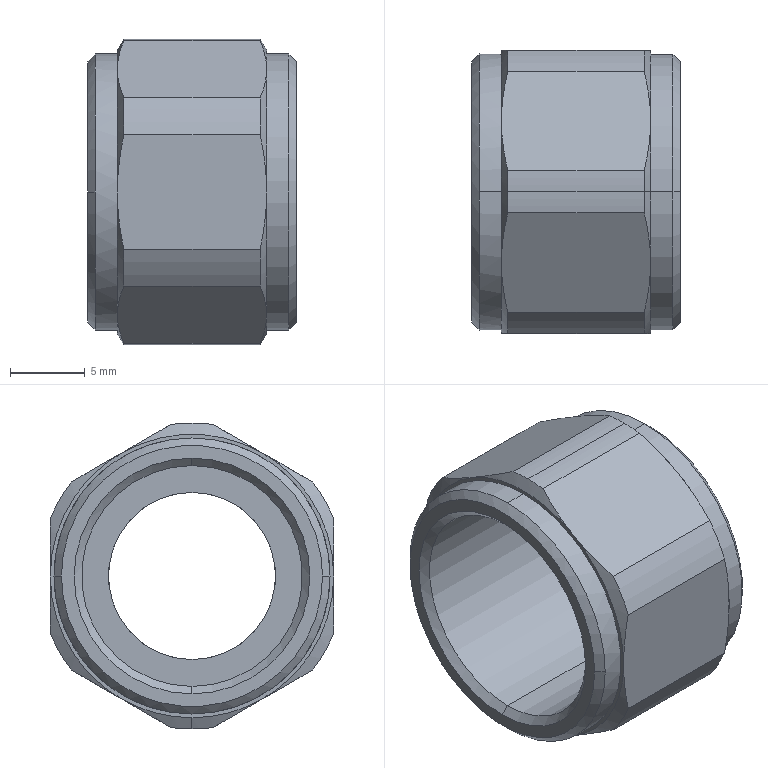Part | STEP file | 7C | 1 solid | 48 faces | box 14 x 19 x 20.5 mm | volume 1922 mm3 | cone 22 | cylinder 15 | plane 11 | commonest cylinder face diameters 20.5 x7 18.5 x4 11.2 x2 14.8 x2
STEP:
#1=CARTESIAN_POINT('',(11.,0.,-7.4));
#2=VERTEX_POINT('',#1);
#3=CARTESIAN_POINT('',(11.,0.,7.4));
#4=VERTEX_POINT('',#3);
#5=CARTESIAN_POINT('',(11.,0.,0.));
#6=DIRECTION('',(-1.,0.,0.));
#7=DIRECTION('',(0.,0.,1.));
#8=AXIS2_PLACEMENT_3D('',#5,#6,#7);
#9=CIRCLE('',#8,7.4);
#10=EDGE_CURVE('',#2,#4,#9,.T.);
#11=ORIENTED_EDGE('',*,*,#10,.F.);
#12=CARTESIAN_POINT('',(0.5,0.,-7.4));
#13=VERTEX_POINT('',#12);
#14=CARTESIAN_POINT('',(-2.908,0.,-7.4));
#15=DIRECTION('',(-1.,0.,0.));
#16=VECTOR('',#15,1000.);
#17=LINE('',#14,#16);
#18=EDGE_CURVE('',#2,#13,#17,.T.);
#19=ORIENTED_EDGE('',*,*,#18,.T.);
#20=CARTESIAN_POINT('',(0.5,0.,7.4));
#21=VERTEX_POINT('',#20);
#22=CARTESIAN_POINT('',(0.5,0.,0.));
#23=DIRECTION('',(1.,0.,0.));
#24=DIRECTION('',(0.,0.,1.));
#25=AXIS2_PLACEMENT_3D('',#22,#23,#24);
#26=CIRCLE('',#25,7.4);
#27=EDGE_CURVE('',#21,#13,#26,.T.);
#28=ORIENTED_EDGE('',*,*,#27,.F.);
#29=CARTESIAN_POINT('',(-2.908,0.,7.4));
#30=DIRECTION('',(-1.,0.,0.));
#31=VECTOR('',#30,1000.);
#32=LINE('',#29,#31);
#33=EDGE_CURVE('',#4,#21,#32,.T.);
#34=ORIENTED_EDGE('',*,*,#33,.F.);
#35=EDGE_LOOP('',(#11,#19,#28,#34));
#36=FACE_OUTER_BOUND('',#35,.T.);
#37=CARTESIAN_POINT('',(-2.908,0.,0.));
#38=DIRECTION('',(-1.,0.,0.));
#39=DIRECTION('',(0.,0.,1.));
#40=AXIS2_PLACEMENT_3D('',#37,#38,#39);
#41=CYLINDRICAL_SURFACE('',#40,7.4);
#42=ADVANCED_FACE('',(#36),#41,.F.);
#43=ORIENTED_EDGE('',*,*,#27,.T.);
#44=CARTESIAN_POINT('',(0.,0.,-7.9));
#45=VERTEX_POINT('',#44);
#46=CARTESIAN_POINT('',(0.,0.,-7.9));
#47=DIRECTION('',(-0.7071,0.,-0.7071));
#48=VECTOR('',#47,1000.);
#49=LINE('',#46,#48);
#50=EDGE_CURVE('',#13,#45,#49,.T.);
#51=ORIENTED_EDGE('',*,*,#50,.T.);
#52=CARTESIAN_POINT('',(0.,0.,7.9));
#53=VERTEX_POINT('',#52);
#54=CARTESIAN_POINT('',(0.,0.,0.));
#55=DIRECTION('',(1.,0.,0.));
#56=DIRECTION('',(0.,0.,1.));
#57=AXIS2_PLACEMENT_3D('',#54,#55,#56);
#58=CIRCLE('',#57,7.9);
#59=EDGE_CURVE('',#53,#45,#58,.T.);
#60=ORIENTED_EDGE('',*,*,#59,.F.);
#61=CARTESIAN_POINT('',(0.,0.,7.9));
#62=DIRECTION('',(-0.7071,0.,0.7071));
#63=VECTOR('',#62,1000.);
#64=LINE('',#61,#63);
#65=EDGE_CURVE('',#21,#53,#64,.T.);
#66=ORIENTED_EDGE('',*,*,#65,.F.);
#67=EDGE_LOOP('',(#43,#51,#60,#66));
#68=FACE_OUTER_BOUND('',#67,.T.);
#69=CARTESIAN_POINT('',(0.,0.,0.));
#70=DIRECTION('',(-1.,0.,0.));
#71=DIRECTION('',(0.,0.,1.));
#72=AXIS2_PLACEMENT_3D('',#69,#70,#71);
#73=CONICAL_SURFACE('',#72,7.9,0.7854);
#74=ADVANCED_FACE('',(#68),#73,.F.);
#75=CARTESIAN_POINT('',(13.5,0.,-5.6));
#76=VERTEX_POINT('',#75);
#77=CARTESIAN_POINT('',(13.5,-5.6,0.));
#78=VERTEX_POINT('',#77);
#79=CARTESIAN_POINT('',(13.5,0.,0.));
#80=DIRECTION('',(-1.,0.,0.));
#81=DIRECTION('',(0.,0.,1.));
#82=AXIS2_PLACEMENT_3D('',#79,#80,#81);
#83=CIRCLE('',#82,5.6);
#84=EDGE_CURVE('',#76,#78,#83,.T.);
#85=ORIENTED_EDGE('',*,*,#84,.F.);
#86=CARTESIAN_POINT('',(11.,0.,-5.6));
#87=VERTEX_POINT('',#86);
#88=CARTESIAN_POINT('',(-2.908,0.,-5.6));
#89=DIRECTION('',(-1.,0.,0.));
#90=VECTOR('',#89,1000.);
#91=LINE('',#88,#90);
#92=EDGE_CURVE('',#76,#87,#91,.T.);
#93=ORIENTED_EDGE('',*,*,#92,.T.);
#94=CARTESIAN_POINT('',(11.,0.,5.6));
#95=VERTEX_POINT('',#94);
#96=CARTESIAN_POINT('',(11.,0.,0.));
#97=DIRECTION('',(1.,0.,0.));
#98=DIRECTION('',(0.,0.,1.));
#99=AXIS2_PLACEMENT_3D('',#96,#97,#98);
#100=CIRCLE('',#99,5.6);
#101=EDGE_CURVE('',#95,#87,#100,.T.);
#102=ORIENTED_EDGE('',*,*,#101,.F.);
#103=CARTESIAN_POINT('',(13.5,0.,5.6));
#104=VERTEX_POINT('',#103);
#105=CARTESIAN_POINT('',(-2.908,0.,5.6));
#106=DIRECTION('',(-1.,0.,0.));
#107=VECTOR('',#106,1000.);
#108=LINE('',#105,#107);
#109=EDGE_CURVE('',#104,#95,#108,.T.);
#110=ORIENTED_EDGE('',*,*,#109,.F.);
#111=CARTESIAN_POINT('',(13.5,0.,0.));
#112=DIRECTION('',(-1.,0.,0.));
#113=DIRECTION('',(0.,0.,1.));
#114=AXIS2_PLACEMENT_3D('',#111,#112,#113);
#115=CIRCLE('',#114,5.6);
#116=EDGE_CURVE('',#78,#104,#115,.T.);
#117=ORIENTED_EDGE('',*,*,#116,.F.);
#118=EDGE_LOOP('',(#85,#93,#102,#110,#117));
#119=FACE_OUTER_BOUND('',#118,.T.);
#120=CARTESIAN_POINT('',(-2.908,0.,0.));
#121=DIRECTION('',(-1.,0.,0.));
#122=DIRECTION('',(0.,0.,1.));
#123=AXIS2_PLACEMENT_3D('',#120,#121,#122);
#124=CYLINDRICAL_SURFACE('',#123,5.6);
#125=ADVANCED_FACE('',(#119),#124,.F.);
#126=CARTESIAN_POINT('',(13.5,5.6,0.));
#127=VERTEX_POINT('',#126);
#128=CARTESIAN_POINT('',(13.5,0.,0.));
#129=DIRECTION('',(-1.,0.,0.));
#130=DIRECTION('',(0.,0.,1.));
#131=AXIS2_PLACEMENT_3D('',#128,#129,#130);
#132=CIRCLE('',#131,5.6);
#133=EDGE_CURVE('',#127,#76,#132,.T.);
#134=ORIENTED_EDGE('',*,*,#133,.T.);
#135=ORIENTED_EDGE('',*,*,#84,.T.);
#136=CARTESIAN_POINT('',(14.,-6.1,0.));
#137=VERTEX_POINT('',#136);
#138=CARTESIAN_POINT('',(14.,-6.1,0.));
#139=DIRECTION('',(0.7071,-0.7071,0.));
#140=VECTOR('',#139,1000.);
#141=LINE('',#138,#140);
#142=EDGE_CURVE('',#78,#137,#141,.T.);
#143=ORIENTED_EDGE('',*,*,#142,.T.);
#144=CARTESIAN_POINT('',(14.,6.1,0.));
#145=VERTEX_POINT('',#144);
#146=CARTESIAN_POINT('',(14.,0.,0.));
#147=DIRECTION('',(-1.,0.,0.));
#148=DIRECTION('',(0.,1.,0.));
#149=AXIS2_PLACEMENT_3D('',#146,#147,#148);
#150=CIRCLE('',#149,6.1);
#151=EDGE_CURVE('',#145,#137,#150,.T.);
#152=ORIENTED_EDGE('',*,*,#151,.F.);
#153=CARTESIAN_POINT('',(14.,6.1,0.));
#154=DIRECTION('',(0.7071,0.7071,0.));
#155=VECTOR('',#154,1000.);
#156=LINE('',#153,#155);
#157=EDGE_CURVE('',#127,#145,#156,.T.);
#158=ORIENTED_EDGE('',*,*,#157,.F.);
#159=EDGE_LOOP('',(#134,#135,#143,#152,#158));
#160=FACE_OUTER_BOUND('',#159,.T.);
#161=CARTESIAN_POINT('',(14.,0.,0.));
#162=DIRECTION('',(1.,0.,0.));
#163=DIRECTION('',(0.,1.,0.));
#164=AXIS2_PLACEMENT_3D('',#161,#162,#163);
#165=CONICAL_SURFACE('',#164,6.1,0.7854);
#166=ADVANCED_FACE('',(#160),#165,.F.);
#167=CARTESIAN_POINT('',(0.,8.75,0.));
#168=VERTEX_POINT('',#167);
#169=CARTESIAN_POINT('',(0.,-8.75,0.));
#170=VERTEX_POINT('',#169);
#171=CARTESIAN_POINT('',(0.,0.,0.));
#172=DIRECTION('',(1.,0.,0.));
#173=DIRECTION('',(0.,1.,0.));
#174=AXIS2_PLACEMENT_3D('',#171,#172,#173);
#175=CIRCLE('',#174,8.75);
#176=EDGE_CURVE('',#168,#170,#175,.T.);
#177=ORIENTED_EDGE('',*,*,#176,.T.);
#178=CARTESIAN_POINT('',(0.5,-9.25,0.));
#179=VERTEX_POINT('',#178);
#180=CARTESIAN_POINT('',(0.5,-9.25,0.));
#181=DIRECTION('',(0.7071,-0.7071,0.));
#182=VECTOR('',#181,1000.);
#183=LINE('',#180,#182);
#184=EDGE_CURVE('',#170,#179,#183,.T.);
#185=ORIENTED_EDGE('',*,*,#184,.T.);
#186=CARTESIAN_POINT('',(0.5,0.,9.25));
#187=VERTEX_POINT('',#186);
#188=CARTESIAN_POINT('',(0.5,0.,0.));
#189=DIRECTION('',(-1.,0.,0.));
#190=DIRECTION('',(0.,0.,-1.));
#191=AXIS2_PLACEMENT_3D('',#188,#189,#190);
#192=CIRCLE('',#191,9.25);
#193=EDGE_CURVE('',#179,#187,#192,.T.);
#194=ORIENTED_EDGE('',*,*,#193,.T.);
#195=CARTESIAN_POINT('',(0.5,9.25,0.));
#196=VERTEX_POINT('',#195);
#197=CARTESIAN_POINT('',(0.5,0.,0.));
#198=DIRECTION('',(-1.,0.,0.));
#199=DIRECTION('',(0.,0.,-1.));
#200=AXIS2_PLACEMENT_3D('',#197,#198,#199);
#201=CIRCLE('',#200,9.25);
#202=EDGE_CURVE('',#187,#196,#201,.T.);
#203=ORIENTED_EDGE('',*,*,#202,.T.);
#204=CARTESIAN_POINT('',(0.5,9.25,0.));
#205=DIRECTION('',(0.7071,0.7071,0.));
#206=VECTOR('',#205,1000.);
#207=LINE('',#204,#206);
#208=EDGE_CURVE('',#168,#196,#207,.T.);
#209=ORIENTED_EDGE('',*,*,#208,.F.);
#210=EDGE_LOOP('',(#177,#185,#194,#203,#209));
#211=FACE_OUTER_BOUND('',#210,.T.);
#212=CARTESIAN_POINT('',(0.5,0.,0.));
#213=DIRECTION('',(1.,0.,0.));
#214=DIRECTION('',(0.,1.,0.));
#215=AXIS2_PLACEMENT_3D('',#212,#213,#214);
#216=CONICAL_SURFACE('',#215,9.25,0.7854);
#217=ADVANCED_FACE('',(#211),#216,.T.);
#218=CARTESIAN_POINT('',(2.,0.,9.25));
#219=VERTEX_POINT('',#218);
#220=CARTESIAN_POINT('',(2.,0.,-9.25));
#221=VERTEX_POINT('',#220);
#222=CARTESIAN_POINT('',(2.,0.,0.));
#223=DIRECTION('',(-1.,0.,0.));
#224=DIRECTION('',(0.,0.,1.));
#225=AXIS2_PLACEMENT_3D('',#222,#223,#224);
#226=CIRCLE('',#225,9.25);
#227=EDGE_CURVE('',#219,#221,#226,.T.);
#228=ORIENTED_EDGE('',*,*,#227,.T.);
#229=CARTESIAN_POINT('',(0.5,0.,-9.25));
#230=VERTEX_POINT('',#229);
#231=CARTESIAN_POINT('',(-2.908,0.,-9.25));
#232=DIRECTION('',(-1.,0.,0.));
#233=VECTOR('',#232,1000.);
#234=LINE('',#231,#233);
#235=EDGE_CURVE('',#221,#230,#234,.T.);
#236=ORIENTED_EDGE('',*,*,#235,.T.);
#237=CARTESIAN_POINT('',(0.5,0.,0.));
#238=DIRECTION('',(-1.,0.,0.));
#239=DIRECTION('',(0.,0.,-1.));
#240=AXIS2_PLACEMENT_3D('',#237,#238,#239);
#241=CIRCLE('',#240,9.25);
#242=EDGE_CURVE('',#196,#230,#241,.T.);
#243=ORIENTED_EDGE('',*,*,#242,.F.);
#244=ORIENTED_EDGE('',*,*,#202,.F.);
#245=CARTESIAN_POINT('',(-2.908,0.,9.25));
#246=DIRECTION('',(-1.,0.,0.));
#247=VECTOR('',#246,1000.);
#248=LINE('',#245,#247);
#249=EDGE_CURVE('',#219,#187,#248,.T.);
#250=ORIENTED_EDGE('',*,*,#249,.F.);
#251=EDGE_LOOP('',(#228,#236,#243,#244,#250));
#252=FACE_OUTER_BOUND('',#251,.T.);
#253=CARTESIAN_POINT('',(-2.908,0.,0.));
#254=DIRECTION('',(-1.,0.,0.));
#255=DIRECTION('',(0.,0.,1.));
#256=AXIS2_PLACEMENT_3D('',#253,#254,#255);
#257=CYLINDRICAL_SURFACE('',#256,9.25);
#258=ADVANCED_FACE('',(#252),#257,.T.);
#259=CARTESIAN_POINT('',(14.,0.,-8.75));
#260=VERTEX_POINT('',#259);
#261=CARTESIAN_POINT('',(14.,0.,8.75));
#262=VERTEX_POINT('',#261);
#263=CARTESIAN_POINT('',(14.,0.,0.));
#264=DIRECTION('',(1.,0.,0.));
#265=DIRECTION('',(0.,0.,1.));
#266=AXIS2_PLACEMENT_3D('',#263,#264,#265);
#267=CIRCLE('',#266,8.75);
#268=EDGE_CURVE('',#260,#262,#267,.T.);
#269=ORIENTED_EDGE('',*,*,#268,.F.);
#270=CARTESIAN_POINT('',(13.5,0.,-9.25));
#271=VERTEX_POINT('',#270);
#272=CARTESIAN_POINT('',(13.5,0.,-9.25));
#273=DIRECTION('',(-0.7071,0.,-0.7071));
#274=VECTOR('',#273,1000.);
#275=LINE('',#272,#274);
#276=EDGE_CURVE('',#260,#271,#275,.T.);
#277=ORIENTED_EDGE('',*,*,#276,.T.);
#278=CARTESIAN_POINT('',(13.5,0.,9.25));
#279=VERTEX_POINT('',#278);
#280=CARTESIAN_POINT('',(13.5,0.,0.));
#281=DIRECTION('',(1.,0.,0.));
#282=DIRECTION('',(0.,0.,1.));
#283=AXIS2_PLACEMENT_3D('',#280,#281,#282);
#284=CIRCLE('',#283,9.25);
#285=EDGE_CURVE('',#271,#279,#284,.T.);
#286=ORIENTED_EDGE('',*,*,#285,.T.);
#287=CARTESIAN_POINT('',(13.5,0.,9.25));
#288=DIRECTION('',(-0.7071,0.,0.7071));
#289=VECTOR('',#288,1000.);
#290=LINE('',#287,#289);
#291=EDGE_CURVE('',#262,#279,#290,.T.);
#292=ORIENTED_EDGE('',*,*,#291,.F.);
#293=EDGE_LOOP('',(#269,#277,#286,#292));
#294=FACE_OUTER_BOUND('',#293,.T.);
#295=CARTESIAN_POINT('',(13.5,0.,0.));
#296=DIRECTION('',(-1.,0.,0.));
#297=DIRECTION('',(0.,0.,1.));
#298=AXIS2_PLACEMENT_3D('',#295,#296,#297);
#299=CONICAL_SURFACE('',#298,9.25,0.7854);
#300=ADVANCED_FACE('',(#294),#299,.T.);
#301=ORIENTED_EDGE('',*,*,#285,.F.);
#302=CARTESIAN_POINT('',(12.,0.,-9.25));
#303=VERTEX_POINT('',#302);
#304=CARTESIAN_POINT('',(-2.908,0.,-9.25));
#305=DIRECTION('',(-1.,0.,0.));
#306=VECTOR('',#305,1000.);
#307=LINE('',#304,#306);
#308=EDGE_CURVE('',#271,#303,#307,.T.);
#309=ORIENTED_EDGE('',*,*,#308,.T.);
#310=CARTESIAN_POINT('',(12.,0.,9.25));
#311=VERTEX_POINT('',#310);
#312=CARTESIAN_POINT('',(12.,0.,0.));
#313=DIRECTION('',(1.,0.,0.));
#314=DIRECTION('',(0.,0.,1.));
#315=AXIS2_PLACEMENT_3D('',#312,#313,#314);
#316=CIRCLE('',#315,9.25);
#317=EDGE_CURVE('',#303,#311,#316,.T.);
#318=ORIENTED_EDGE('',*,*,#317,.T.);
#319=CARTESIAN_POINT('',(-2.908,0.,9.25));
#320=DIRECTION('',(-1.,0.,0.));
#321=VECTOR('',#320,1000.);
#322=LINE('',#319,#321);
#323=EDGE_CURVE('',#279,#311,#322,.T.);
#324=ORIENTED_EDGE('',*,*,#323,.F.);
#325=EDGE_LOOP('',(#301,#309,#318,#324));
#326=FACE_OUTER_BOUND('',#325,.T.);
#327=CARTESIAN_POINT('',(-2.908,0.,0.));
#328=DIRECTION('',(-1.,0.,0.));
#329=DIRECTION('',(0.,0.,1.));
#330=AXIS2_PLACEMENT_3D('',#327,#328,#329);
#331=CYLINDRICAL_SURFACE('',#330,9.25);
#332=ADVANCED_FACE('',(#326),#331,.T.);
#333=CARTESIAN_POINT('',(2.,0.,-9.5));
#334=VERTEX_POINT('',#333);
#335=CARTESIAN_POINT('',(2.,-4.75,-8.227));
#336=VERTEX_POINT('',#335);
#337=CARTESIAN_POINT('',(2.,0.,0.));
#338=DIRECTION('',(-1.,0.,0.));
#339=DIRECTION('',(0.,0.,-1.));
#340=AXIS2_PLACEMENT_3D('',#337,#338,#339);
#341=CIRCLE('',#340,9.5);
#342=EDGE_CURVE('',#334,#336,#341,.T.);
#343=ORIENTED_EDGE('',*,*,#342,.F.);
#344=CARTESIAN_POINT('',(2.433,0.,-10.25));
#345=VERTEX_POINT('',#344);
#346=CARTESIAN_POINT('',(2.433,0.,-10.25));
#347=DIRECTION('',(0.5,0.,-0.866));
#348=VECTOR('',#347,1000.);
#349=LINE('',#346,#348);
#350=EDGE_CURVE('',#334,#345,#349,.T.);
#351=ORIENTED_EDGE('',*,*,#350,.T.);
#352=CARTESIAN_POINT('',(2.433,-1.417,-10.152));
#353=VERTEX_POINT('',#352);
#354=CARTESIAN_POINT('',(2.433,0.,0.));
#355=DIRECTION('',(1.,0.,0.));
#356=DIRECTION('',(0.,0.,1.));
#357=AXIS2_PLACEMENT_3D('',#354,#355,#356);
#358=CIRCLE('',#357,10.25);
#359=EDGE_CURVE('',#353,#345,#358,.T.);
#360=ORIENTED_EDGE('',*,*,#359,.F.);
#361=CARTESIAN_POINT('',(2.433,-1.417,-10.152));
#362=CARTESIAN_POINT('',(2.158,-2.515,-9.517));
#363=CARTESIAN_POINT('',(2.,-3.625,-8.877));
#364=CARTESIAN_POINT('',(2.,-4.75,-8.227));
#365=B_SPLINE_CURVE_WITH_KNOTS('',3,(#361,#362,#363,#364),.UNSPECIFIED.,.F.,.F.,(4,4),(0.,0.003873),.UNSPECIFIED.);
#366=EDGE_CURVE('',#353,#336,#365,.T.);
#367=ORIENTED_EDGE('',*,*,#366,.T.);
#368=EDGE_LOOP('',(#343,#351,#360,#367));
#369=FACE_OUTER_BOUND('',#368,.T.);
#370=CARTESIAN_POINT('',(2.433,0.,0.));
#371=DIRECTION('',(1.,0.,0.));
#372=DIRECTION('',(0.,0.,-1.));
#373=AXIS2_PLACEMENT_3D('',#370,#371,#372);
#374=CONICAL_SURFACE('',#373,10.25,1.047);
#375=ADVANCED_FACE('',(#369),#374,.T.);
#376=CARTESIAN_POINT('',(12.,0.,9.5));
#377=VERTEX_POINT('',#376);
#378=CARTESIAN_POINT('',(12.,-4.75,8.227));
#379=VERTEX_POINT('',#378);
#380=CARTESIAN_POINT('',(12.,0.,0.));
#381=DIRECTION('',(1.,0.,0.));
#382=DIRECTION('',(0.,0.,1.));
#383=AXIS2_PLACEMENT_3D('',#380,#381,#382);
#384=CIRCLE('',#383,9.5);
#385=EDGE_CURVE('',#377,#379,#384,.T.);
#386=ORIENTED_EDGE('',*,*,#385,.F.);
#387=CARTESIAN_POINT('',(11.567,0.,10.25));
#388=VERTEX_POINT('',#387);
#389=CARTESIAN_POINT('',(11.567,0.,10.25));
#390=DIRECTION('',(-0.5,0.,0.866));
#391=VECTOR('',#390,1000.);
#392=LINE('',#389,#391);
#393=EDGE_CURVE('',#377,#388,#392,.T.);
#394=ORIENTED_EDGE('',*,*,#393,.T.);
#395=CARTESIAN_POINT('',(11.567,-1.417,10.152));
#396=VERTEX_POINT('',#395);
#397=CARTESIAN_POINT('',(11.567,0.,0.));
#398=DIRECTION('',(1.,0.,0.));
#399=DIRECTION('',(0.,0.,1.));
#400=AXIS2_PLACEMENT_3D('',#397,#398,#399);
#401=CIRCLE('',#400,10.25);
#402=EDGE_CURVE('',#388,#396,#401,.T.);
#403=ORIENTED_EDGE('',*,*,#402,.T.);
#404=CARTESIAN_POINT('',(11.567,-1.417,10.152));
#405=CARTESIAN_POINT('',(11.842,-2.515,9.517));
#406=CARTESIAN_POINT('',(12.,-3.625,8.877));
#407=CARTESIAN_POINT('',(12.,-4.75,8.227));
#408=B_SPLINE_CURVE_WITH_KNOTS('',3,(#404,#405,#406,#407),.UNSPECIFIED.,.F.,.F.,(4,4),(0.,0.003873),.UNSPECIFIED.);
#409=EDGE_CURVE('',#396,#379,#408,.T.);
#410=ORIENTED_EDGE('',*,*,#409,.T.);
#411=EDGE_LOOP('',(#386,#394,#403,#410));
#412=FACE_OUTER_BOUND('',#411,.T.);
#413=CARTESIAN_POINT('',(11.567,0.,0.));
#414=DIRECTION('',(-1.,0.,0.));
#415=DIRECTION('',(0.,0.,1.));
#416=AXIS2_PLACEMENT_3D('',#413,#414,#415);
#417=CONICAL_SURFACE('',#416,10.25,1.047);
#418=ADVANCED_FACE('',(#412),#417,.T.);
#419=ORIENTED_EDGE('',*,*,#402,.F.);
#420=CARTESIAN_POINT('',(2.433,0.,10.25));
#421=VERTEX_POINT('',#420);
#422=CARTESIAN_POINT('',(-2.908,0.,10.25));
#423=DIRECTION('',(-1.,0.,0.));
#424=VECTOR('',#423,1000.);
#425=LINE('',#422,#424);
#426=EDGE_CURVE('',#388,#421,#425,.T.);
#427=ORIENTED_EDGE('',*,*,#426,.T.);
#428=CARTESIAN_POINT('',(2.433,-1.417,10.152));
#429=VERTEX_POINT('',#428);
#430=CARTESIAN_POINT('',(2.433,0.,0.));
#431=DIRECTION('',(1.,0.,0.));
#432=DIRECTION('',(0.,0.,1.));
#433=AXIS2_PLACEMENT_3D('',#430,#431,#432);
#434=CIRCLE('',#433,10.25);
#435=EDGE_CURVE('',#421,#429,#434,.T.);
#436=ORIENTED_EDGE('',*,*,#435,.T.);
#437=CARTESIAN_POINT('',(14.,-1.417,10.152));
#438=DIRECTION('',(1.,0.,0.));
#439=VECTOR('',#438,1000.);
#440=LINE('',#437,#439);
#441=EDGE_CURVE('',#429,#396,#440,.T.);
#442=ORIENTED_EDGE('',*,*,#441,.T.);
#443=EDGE_LOOP('',(#419,#427,#436,#442));
#444=FACE_OUTER_BOUND('',#443,.T.);
#445=CARTESIAN_POINT('',(-2.908,0.,0.));
#446=DIRECTION('',(-1.,0.,0.));
#447=DIRECTION('',(0.,0.,1.));
#448=AXIS2_PLACEMENT_3D('',#445,#446,#447);
#449=CYLINDRICAL_SURFACE('',#448,10.25);
#450=ADVANCED_FACE('',(#444),#449,.T.);
#451=ORIENTED_EDGE('',*,*,#18,.F.);
#452=CARTESIAN_POINT('',(11.,0.,0.));
#453=DIRECTION('',(-1.,0.,0.));
#454=DIRECTION('',(0.,0.,1.));
#455=AXIS2_PLACEMENT_3D('',#452,#453,#454);
#456=CIRCLE('',#455,7.4);
#457=EDGE_CURVE('',#4,#2,#456,.T.);
#458=ORIENTED_EDGE('',*,*,#457,.F.);
#459=ORIENTED_EDGE('',*,*,#33,.T.);
#460=CARTESIAN_POINT('',(0.5,0.,0.));
#461=DIRECTION('',(1.,0.,0.));
#462=DIRECTION('',(0.,0.,1.));
#463=AXIS2_PLACEMENT_3D('',#460,#461,#462);
#464=CIRCLE('',#463,7.4);
#465=EDGE_CURVE('',#13,#21,#464,.T.);
#466=ORIENTED_EDGE('',*,*,#465,.F.);
#467=EDGE_LOOP('',(#451,#458,#459,#466));
#468=FACE_OUTER_BOUND('',#467,.T.);
#469=CARTESIAN_POINT('',(-2.908,0.,0.));
#470=DIRECTION('',(-1.,0.,0.));
#471=DIRECTION('',(0.,0.,1.));
#472=AXIS2_PLACEMENT_3D('',#469,#470,#471);
#473=CYLINDRICAL_SURFACE('',#472,7.4);
#474=ADVANCED_FACE('',(#468),#473,.F.);
#475=ORIENTED_EDGE('',*,*,#101,.T.);
#476=CARTESIAN_POINT('',(11.,0.,0.));
#477=DIRECTION('',(1.,0.,0.));
#478=DIRECTION('',(0.,0.,1.));
#479=AXIS2_PLACEMENT_3D('',#476,#477,#478);
#480=CIRCLE('',#479,5.6);
#481=EDGE_CURVE('',#87,#95,#480,.T.);
#482=ORIENTED_EDGE('',*,*,#481,.T.);
#483=EDGE_LOOP('',(#475,#482));
#484=FACE_BOUND('',#483,.T.);
#485=ORIENTED_EDGE('',*,*,#457,.T.);
#486=ORIENTED_EDGE('',*,*,#10,.T.);
#487=EDGE_LOOP('',(#485,#486));
#488=FACE_OUTER_BOUND('',#487,.T.);
#489=CARTESIAN_POINT('',(11.,0.,-7.4));
#490=DIRECTION('',(-1.,0.,0.));
#491=DIRECTION('',(0.,0.,1.));
#492=AXIS2_PLACEMENT_3D('',#489,#490,#491);
#493=PLANE('',#492);
#494=ADVANCED_FACE('',(#484,#488),#493,.T.);
#495=ORIENTED_EDGE('',*,*,#50,.F.);
#496=ORIENTED_EDGE('',*,*,#465,.T.);
#497=ORIENTED_EDGE('',*,*,#65,.T.);
#498=CARTESIAN_POINT('',(0.,0.,0.));
#499=DIRECTION('',(1.,0.,0.));
#500=DIRECTION('',(0.,0.,1.));
#501=AXIS2_PLACEMENT_3D('',#498,#499,#500);
#502=CIRCLE('',#501,7.9);
#503=EDGE_CURVE('',#45,#53,#502,.T.);
#504=ORIENTED_EDGE('',*,*,#503,.F.);
#505=EDGE_LOOP('',(#495,#496,#497,#504));
#506=FACE_OUTER_BOUND('',#505,.T.);
#507=CARTESIAN_POINT('',(0.,0.,0.));
#508=DIRECTION('',(-1.,0.,0.));
#509=DIRECTION('',(0.,0.,1.));
#510=AXIS2_PLACEMENT_3D('',#507,#508,#509);
#511=CONICAL_SURFACE('',#510,7.9,0.7854);
#512=ADVANCED_FACE('',(#506),#511,.F.);
#513=ORIENTED_EDGE('',*,*,#92,.F.);
#514=ORIENTED_EDGE('',*,*,#133,.F.);
#515=CARTESIAN_POINT('',(13.5,0.,0.));
#516=DIRECTION('',(-1.,0.,0.));
#517=DIRECTION('',(0.,0.,1.));
#518=AXIS2_PLACEMENT_3D('',#515,#516,#517);
#519=CIRCLE('',#518,5.6);
#520=EDGE_CURVE('',#104,#127,#519,.T.);
#521=ORIENTED_EDGE('',*,*,#520,.F.);
#522=ORIENTED_EDGE('',*,*,#109,.T.);
#523=ORIENTED_EDGE('',*,*,#481,.F.);
#524=EDGE_LOOP('',(#513,#514,#521,#522,#523));
#525=FACE_OUTER_BOUND('',#524,.T.);
#526=CARTESIAN_POINT('',(-2.908,0.,0.));
#527=DIRECTION('',(-1.,0.,0.));
#528=DIRECTION('',(0.,0.,1.));
#529=AXIS2_PLACEMENT_3D('',#526,#527,#528);
#530=CYLINDRICAL_SURFACE('',#529,5.6);
#531=ADVANCED_FACE('',(#525),#530,.F.);
#532=ORIENTED_EDGE('',*,*,#59,.T.);
#533=ORIENTED_EDGE('',*,*,#503,.T.);
#534=EDGE_LOOP('',(#532,#533));
#535=FACE_BOUND('',#534,.T.);
#536=ORIENTED_EDGE('',*,*,#176,.F.);
#537=CARTESIAN_POINT('',(0.,0.,0.));
#538=DIRECTION('',(1.,0.,0.));
#539=DIRECTION('',(0.,1.,0.));
#540=AXIS2_PLACEMENT_3D('',#537,#538,#539);
#541=CIRCLE('',#540,8.75);
#542=EDGE_CURVE('',#170,#168,#541,.T.);
#543=ORIENTED_EDGE('',*,*,#542,.F.);
#544=EDGE_LOOP('',(#536,#543));
#545=FACE_OUTER_BOUND('',#544,.T.);
#546=CARTESIAN_POINT('',(0.,0.,-10.97));
#547=DIRECTION('',(1.,0.,0.));
#548=DIRECTION('',(0.,0.,-1.));
#549=AXIS2_PLACEMENT_3D('',#546,#547,#548);
#550=PLANE('',#549);
#551=ADVANCED_FACE('',(#535,#545),#550,.F.);
#552=ORIENTED_EDGE('',*,*,#142,.F.);
#553=ORIENTED_EDGE('',*,*,#116,.T.);
#554=ORIENTED_EDGE('',*,*,#520,.T.);
#555=ORIENTED_EDGE('',*,*,#157,.T.);
#556=CARTESIAN_POINT('',(14.,0.,0.));
#557=DIRECTION('',(-1.,0.,0.));
#558=DIRECTION('',(0.,1.,0.));
#559=AXIS2_PLACEMENT_3D('',#556,#557,#558);
#560=CIRCLE('',#559,6.1);
#561=EDGE_CURVE('',#137,#145,#560,.T.);
#562=ORIENTED_EDGE('',*,*,#561,.F.);
#563=EDGE_LOOP('',(#552,#553,#554,#555,#562));
#564=FACE_OUTER_BOUND('',#563,.T.);
#565=CARTESIAN_POINT('',(14.,0.,0.));
#566=DIRECTION('',(1.,0.,0.));
#567=DIRECTION('',(0.,1.,0.));
#568=AXIS2_PLACEMENT_3D('',#565,#566,#567);
#569=CONICAL_SURFACE('',#568,6.1,0.7854);
#570=ADVANCED_FACE('',(#564),#569,.F.);
#571=ORIENTED_EDGE('',*,*,#184,.F.);
#572=ORIENTED_EDGE('',*,*,#542,.T.);
#573=ORIENTED_EDGE('',*,*,#208,.T.);
#574=ORIENTED_EDGE('',*,*,#242,.T.);
#575=CARTESIAN_POINT('',(0.5,0.,0.));
#576=DIRECTION('',(-1.,0.,0.));
#577=DIRECTION('',(0.,0.,-1.));
#578=AXIS2_PLACEMENT_3D('',#575,#576,#577);
#579=CIRCLE('',#578,9.25);
#580=EDGE_CURVE('',#230,#179,#579,.T.);
#581=ORIENTED_EDGE('',*,*,#580,.T.);
#582=EDGE_LOOP('',(#571,#572,#573,#574,#581));
#583=FACE_OUTER_BOUND('',#582,.T.);
#584=CARTESIAN_POINT('',(0.5,0.,0.));
#585=DIRECTION('',(1.,0.,0.));
#586=DIRECTION('',(0.,1.,0.));
#587=AXIS2_PLACEMENT_3D('',#584,#585,#586);
#588=CONICAL_SURFACE('',#587,9.25,0.7854);
#589=ADVANCED_FACE('',(#583),#588,.T.);
#590=CARTESIAN_POINT('',(14.,0.,0.));
#591=DIRECTION('',(1.,0.,0.));
#592=DIRECTION('',(0.,0.,1.));
#593=AXIS2_PLACEMENT_3D('',#590,#591,#592);
#594=CIRCLE('',#593,8.75);
#595=EDGE_CURVE('',#262,#260,#594,.T.);
#596=ORIENTED_EDGE('',*,*,#595,.T.);
#597=ORIENTED_EDGE('',*,*,#268,.T.);
#598=EDGE_LOOP('',(#596,#597));
#599=FACE_OUTER_BOUND('',#598,.T.);
#600=ORIENTED_EDGE('',*,*,#151,.T.);
#601=ORIENTED_EDGE('',*,*,#561,.T.);
#602=EDGE_LOOP('',(#600,#601));
#603=FACE_BOUND('',#602,.T.);
#604=CARTESIAN_POINT('',(14.,0.,-10.97));
#605=DIRECTION('',(1.,0.,0.));
#606=DIRECTION('',(0.,0.,-1.));
#607=AXIS2_PLACEMENT_3D('',#604,#605,#606);
#608=PLANE('',#607);
#609=ADVANCED_FACE('',(#599,#603),#608,.T.);
#610=ORIENTED_EDGE('',*,*,#235,.F.);
#611=CARTESIAN_POINT('',(2.,0.,0.));
#612=DIRECTION('',(-1.,0.,0.));
#613=DIRECTION('',(0.,0.,1.));
#614=AXIS2_PLACEMENT_3D('',#611,#612,#613);
#615=CIRCLE('',#614,9.25);
#616=EDGE_CURVE('',#221,#219,#615,.T.);
#617=ORIENTED_EDGE('',*,*,#616,.T.);
#618=ORIENTED_EDGE('',*,*,#249,.T.);
#619=ORIENTED_EDGE('',*,*,#193,.F.);
#620=ORIENTED_EDGE('',*,*,#580,.F.);
#621=EDGE_LOOP('',(#610,#617,#618,#619,#620));
#622=FACE_OUTER_BOUND('',#621,.T.);
#623=CARTESIAN_POINT('',(-2.908,0.,0.));
#624=DIRECTION('',(-1.,0.,0.));
#625=DIRECTION('',(0.,0.,1.));
#626=AXIS2_PLACEMENT_3D('',#623,#624,#625);
#627=CYLINDRICAL_SURFACE('',#626,9.25);
#628=ADVANCED_FACE('',(#622),#627,.T.);
#629=ORIENTED_EDGE('',*,*,#276,.F.);
#630=ORIENTED_EDGE('',*,*,#595,.F.);
#631=ORIENTED_EDGE('',*,*,#291,.T.);
#632=CARTESIAN_POINT('',(13.5,0.,0.));
#633=DIRECTION('',(1.,0.,0.));
#634=DIRECTION('',(0.,0.,1.));
#635=AXIS2_PLACEMENT_3D('',#632,#633,#634);
#636=CIRCLE('',#635,9.25);
#637=EDGE_CURVE('',#279,#271,#636,.T.);
#638=ORIENTED_EDGE('',*,*,#637,.T.);
#639=EDGE_LOOP('',(#629,#630,#631,#638));
#640=FACE_OUTER_BOUND('',#639,.T.);
#641=CARTESIAN_POINT('',(13.5,0.,0.));
#642=DIRECTION('',(-1.,0.,0.));
#643=DIRECTION('',(0.,0.,1.));
#644=AXIS2_PLACEMENT_3D('',#641,#642,#643);
#645=CONICAL_SURFACE('',#644,9.25,0.7854);
#646=ADVANCED_FACE('',(#640),#645,.T.);
#647=ORIENTED_EDGE('',*,*,#227,.F.);
#648=ORIENTED_EDGE('',*,*,#616,.F.);
#649=EDGE_LOOP('',(#647,#648));
#650=FACE_BOUND('',#649,.T.);
#651=CARTESIAN_POINT('',(2.,-9.5,0.));
#652=VERTEX_POINT('',#651);
#653=CARTESIAN_POINT('',(2.,-4.75,8.227));
#654=VERTEX_POINT('',#653);
#655=CARTESIAN_POINT('',(2.,0.,0.));
#656=DIRECTION('',(-1.,0.,0.));
#657=DIRECTION('',(0.,0.,-1.));
#658=AXIS2_PLACEMENT_3D('',#655,#656,#657);
#659=CIRCLE('',#658,9.5);
#660=EDGE_CURVE('',#652,#654,#659,.T.);
#661=ORIENTED_EDGE('',*,*,#660,.T.);
#662=CARTESIAN_POINT('',(2.,4.75,8.227));
#663=VERTEX_POINT('',#662);
#664=CARTESIAN_POINT('',(2.,0.,0.));
#665=DIRECTION('',(-1.,0.,0.));
#666=DIRECTION('',(0.,0.,-1.));
#667=AXIS2_PLACEMENT_3D('',#664,#665,#666);
#668=CIRCLE('',#667,9.5);
#669=EDGE_CURVE('',#654,#663,#668,.T.);
#670=ORIENTED_EDGE('',*,*,#669,.T.);
#671=CARTESIAN_POINT('',(2.,9.5,0.));
#672=VERTEX_POINT('',#671);
#673=CARTESIAN_POINT('',(2.,0.,0.));
#674=DIRECTION('',(-1.,0.,0.));
#675=DIRECTION('',(0.,0.,-1.));
#676=AXIS2_PLACEMENT_3D('',#673,#674,#675);
#677=CIRCLE('',#676,9.5);
#678=EDGE_CURVE('',#663,#672,#677,.T.);
#679=ORIENTED_EDGE('',*,*,#678,.T.);
#680=CARTESIAN_POINT('',(2.,4.75,-8.227));
#681=VERTEX_POINT('',#680);
#682=CARTESIAN_POINT('',(2.,0.,0.));
#683=DIRECTION('',(-1.,0.,0.));
#684=DIRECTION('',(0.,0.,-1.));
#685=AXIS2_PLACEMENT_3D('',#682,#683,#684);
#686=CIRCLE('',#685,9.5);
#687=EDGE_CURVE('',#672,#681,#686,.T.);
#688=ORIENTED_EDGE('',*,*,#687,.T.);
#689=CARTESIAN_POINT('',(2.,0.,0.));
#690=DIRECTION('',(-1.,0.,0.));
#691=DIRECTION('',(0.,0.,-1.));
#692=AXIS2_PLACEMENT_3D('',#689,#690,#691);
#693=CIRCLE('',#692,9.5);
#694=EDGE_CURVE('',#681,#334,#693,.T.);
#695=ORIENTED_EDGE('',*,*,#694,.T.);
#696=ORIENTED_EDGE('',*,*,#342,.T.);
#697=CARTESIAN_POINT('',(2.,0.,0.));
#698=DIRECTION('',(-1.,0.,0.));
#699=DIRECTION('',(0.,0.,-1.));
#700=AXIS2_PLACEMENT_3D('',#697,#698,#699);
#701=CIRCLE('',#700,9.5);
#702=EDGE_CURVE('',#336,#652,#701,.T.);
#703=ORIENTED_EDGE('',*,*,#702,.T.);
#704=EDGE_LOOP('',(#661,#670,#679,#688,#695,#696,#703));
#705=FACE_OUTER_BOUND('',#704,.T.);
#706=CARTESIAN_POINT('',(2.,0.,-9.25));
#707=DIRECTION('',(-1.,0.,0.));
#708=DIRECTION('',(0.,0.,1.));
#709=AXIS2_PLACEMENT_3D('',#706,#707,#708);
#710=PLANE('',#709);
#711=ADVANCED_FACE('',(#650,#705),#710,.T.);
#712=ORIENTED_EDGE('',*,*,#308,.F.);
#713=ORIENTED_EDGE('',*,*,#637,.F.);
#714=ORIENTED_EDGE('',*,*,#323,.T.);
#715=CARTESIAN_POINT('',(12.,0.,0.));
#716=DIRECTION('',(1.,0.,0.));
#717=DIRECTION('',(0.,0.,1.));
#718=AXIS2_PLACEMENT_3D('',#715,#716,#717);
#719=CIRCLE('',#718,9.25);
#720=EDGE_CURVE('',#311,#303,#719,.T.);
#721=ORIENTED_EDGE('',*,*,#720,.T.);
#722=EDGE_LOOP('',(#712,#713,#714,#721));
#723=FACE_OUTER_BOUND('',#722,.T.);
#724=CARTESIAN_POINT('',(-2.908,0.,0.));
#725=DIRECTION('',(-1.,0.,0.));
#726=DIRECTION('',(0.,0.,1.));
#727=AXIS2_PLACEMENT_3D('',#724,#725,#726);
#728=CYLINDRICAL_SURFACE('',#727,9.25);
#729=ADVANCED_FACE('',(#723),#728,.T.);
#730=CARTESIAN_POINT('',(2.433,1.417,10.152));
#731=VERTEX_POINT('',#730);
#732=CARTESIAN_POINT('',(2.433,0.,0.));
#733=DIRECTION('',(1.,0.,0.));
#734=DIRECTION('',(0.,0.,1.));
#735=AXIS2_PLACEMENT_3D('',#732,#733,#734);
#736=CIRCLE('',#735,10.25);
#737=EDGE_CURVE('',#731,#421,#736,.T.);
#738=ORIENTED_EDGE('',*,*,#737,.F.);
#739=CARTESIAN_POINT('',(2.433,1.417,10.152));
#740=CARTESIAN_POINT('',(2.158,2.515,9.517));
#741=CARTESIAN_POINT('',(2.,3.625,8.877));
#742=CARTESIAN_POINT('',(2.,4.75,8.227));
#743=B_SPLINE_CURVE_WITH_KNOTS('',3,(#739,#740,#741,#742),.UNSPECIFIED.,.F.,.F.,(4,4),(0.,0.003873),.UNSPECIFIED.);
#744=EDGE_CURVE('',#731,#663,#743,.T.);
#745=ORIENTED_EDGE('',*,*,#744,.T.);
#746=ORIENTED_EDGE('',*,*,#669,.F.);
#747=CARTESIAN_POINT('',(2.,-4.75,8.227));
#748=CARTESIAN_POINT('',(2.,-3.625,8.877));
#749=CARTESIAN_POINT('',(2.158,-2.515,9.517));
#750=CARTESIAN_POINT('',(2.433,-1.417,10.152));
#751=B_SPLINE_CURVE_WITH_KNOTS('',3,(#747,#748,#749,#750),.UNSPECIFIED.,.F.,.F.,(4,4),(0.,0.003873),.UNSPECIFIED.);
#752=EDGE_CURVE('',#654,#429,#751,.T.);
#753=ORIENTED_EDGE('',*,*,#752,.T.);
#754=ORIENTED_EDGE('',*,*,#435,.F.);
#755=EDGE_LOOP('',(#738,#745,#746,#753,#754));
#756=FACE_OUTER_BOUND('',#755,.T.);
#757=CARTESIAN_POINT('',(2.433,0.,0.));
#758=DIRECTION('',(1.,0.,0.));
#759=DIRECTION('',(0.,0.,-1.));
#760=AXIS2_PLACEMENT_3D('',#757,#758,#759);
#761=CONICAL_SURFACE('',#760,10.25,1.047);
#762=ADVANCED_FACE('',(#756),#761,.T.);
#763=CARTESIAN_POINT('',(2.433,-9.5,3.849));
#764=VERTEX_POINT('',#763);
#765=CARTESIAN_POINT('',(2.,-9.5,0.));
#766=CARTESIAN_POINT('',(2.,-9.5,1.299));
#767=CARTESIAN_POINT('',(2.158,-9.5,2.58));
#768=CARTESIAN_POINT('',(2.433,-9.5,3.849));
#769=B_SPLINE_CURVE_WITH_KNOTS('',3,(#765,#766,#767,#768),.UNSPECIFIED.,.F.,.F.,(4,4),(0.,0.003873),.UNSPECIFIED.);
#770=EDGE_CURVE('',#652,#764,#769,.T.);
#771=ORIENTED_EDGE('',*,*,#770,.T.);
#772=CARTESIAN_POINT('',(2.433,-8.083,6.303));
#773=VERTEX_POINT('',#772);
#774=CARTESIAN_POINT('',(2.433,0.,0.));
#775=DIRECTION('',(-1.,0.,0.));
#776=DIRECTION('',(0.,0.,-1.));
#777=AXIS2_PLACEMENT_3D('',#774,#775,#776);
#778=CIRCLE('',#777,10.25);
#779=EDGE_CURVE('',#764,#773,#778,.T.);
#780=ORIENTED_EDGE('',*,*,#779,.T.);
#781=CARTESIAN_POINT('',(2.433,-8.083,6.303));
#782=CARTESIAN_POINT('',(2.158,-6.985,6.937));
#783=CARTESIAN_POINT('',(2.,-5.875,7.578));
#784=CARTESIAN_POINT('',(2.,-4.75,8.227));
#785=B_SPLINE_CURVE_WITH_KNOTS('',3,(#781,#782,#783,#784),.UNSPECIFIED.,.F.,.F.,(4,4),(0.,0.003873),.UNSPECIFIED.);
#786=EDGE_CURVE('',#773,#654,#785,.T.);
#787=ORIENTED_EDGE('',*,*,#786,.T.);
#788=ORIENTED_EDGE('',*,*,#660,.F.);
#789=EDGE_LOOP('',(#771,#780,#787,#788));
#790=FACE_OUTER_BOUND('',#789,.T.);
#791=CARTESIAN_POINT('',(2.433,0.,0.));
#792=DIRECTION('',(1.,0.,0.));
#793=DIRECTION('',(0.,0.,-1.));
#794=AXIS2_PLACEMENT_3D('',#791,#792,#793);
#795=CONICAL_SURFACE('',#794,10.25,1.047);
#796=ADVANCED_FACE('',(#790),#795,.T.);
#797=CARTESIAN_POINT('',(2.433,-9.5,-3.849));
#798=VERTEX_POINT('',#797);
#799=CARTESIAN_POINT('',(2.433,-9.5,-3.849));
#800=CARTESIAN_POINT('',(2.158,-9.5,-2.58));
#801=CARTESIAN_POINT('',(2.,-9.5,-1.299));
#802=CARTESIAN_POINT('',(2.,-9.5,0.));
#803=B_SPLINE_CURVE_WITH_KNOTS('',3,(#799,#800,#801,#802),.UNSPECIFIED.,.F.,.F.,(4,4),(0.,0.003873),.UNSPECIFIED.);
#804=EDGE_CURVE('',#798,#652,#803,.T.);
#805=ORIENTED_EDGE('',*,*,#804,.T.);
#806=ORIENTED_EDGE('',*,*,#702,.F.);
#807=CARTESIAN_POINT('',(2.433,-8.083,-6.303));
#808=VERTEX_POINT('',#807);
#809=CARTESIAN_POINT('',(2.,-4.75,-8.227));
#810=CARTESIAN_POINT('',(2.,-5.875,-7.578));
#811=CARTESIAN_POINT('',(2.158,-6.985,-6.937));
#812=CARTESIAN_POINT('',(2.433,-8.083,-6.303));
#813=B_SPLINE_CURVE_WITH_KNOTS('',3,(#809,#810,#811,#812),.UNSPECIFIED.,.F.,.F.,(4,4),(0.,0.003873),.UNSPECIFIED.);
#814=EDGE_CURVE('',#336,#808,#813,.T.);
#815=ORIENTED_EDGE('',*,*,#814,.T.);
#816=CARTESIAN_POINT('',(2.433,0.,0.));
#817=DIRECTION('',(-1.,0.,0.));
#818=DIRECTION('',(0.,0.,-1.));
#819=AXIS2_PLACEMENT_3D('',#816,#817,#818);
#820=CIRCLE('',#819,10.25);
#821=EDGE_CURVE('',#808,#798,#820,.T.);
#822=ORIENTED_EDGE('',*,*,#821,.T.);
#823=EDGE_LOOP('',(#805,#806,#815,#822));
#824=FACE_OUTER_BOUND('',#823,.T.);
#825=CARTESIAN_POINT('',(2.433,0.,0.));
#826=DIRECTION('',(1.,0.,0.));
#827=DIRECTION('',(0.,0.,-1.));
#828=AXIS2_PLACEMENT_3D('',#825,#826,#827);
#829=CONICAL_SURFACE('',#828,10.25,1.047);
#830=ADVANCED_FACE('',(#824),#829,.T.);
#831=ORIENTED_EDGE('',*,*,#350,.F.);
#832=ORIENTED_EDGE('',*,*,#694,.F.);
#833=CARTESIAN_POINT('',(2.433,1.417,-10.152));
#834=VERTEX_POINT('',#833);
#835=CARTESIAN_POINT('',(2.,4.75,-8.227));
#836=CARTESIAN_POINT('',(2.,3.625,-8.877));
#837=CARTESIAN_POINT('',(2.158,2.515,-9.517));
#838=CARTESIAN_POINT('',(2.433,1.417,-10.152));
#839=B_SPLINE_CURVE_WITH_KNOTS('',3,(#835,#836,#837,#838),.UNSPECIFIED.,.F.,.F.,(4,4),(0.,0.003873),.UNSPECIFIED.);
#840=EDGE_CURVE('',#681,#834,#839,.T.);
#841=ORIENTED_EDGE('',*,*,#840,.T.);
#842=CARTESIAN_POINT('',(2.433,0.,0.));
#843=DIRECTION('',(1.,0.,0.));
#844=DIRECTION('',(0.,0.,1.));
#845=AXIS2_PLACEMENT_3D('',#842,#843,#844);
#846=CIRCLE('',#845,10.25);
#847=EDGE_CURVE('',#345,#834,#846,.T.);
#848=ORIENTED_EDGE('',*,*,#847,.F.);
#849=EDGE_LOOP('',(#831,#832,#841,#848));
#850=FACE_OUTER_BOUND('',#849,.T.);
#851=CARTESIAN_POINT('',(2.433,0.,0.));
#852=DIRECTION('',(1.,0.,0.));
#853=DIRECTION('',(0.,0.,-1.));
#854=AXIS2_PLACEMENT_3D('',#851,#852,#853);
#855=CONICAL_SURFACE('',#854,10.25,1.047);
#856=ADVANCED_FACE('',(#850),#855,.T.);
#857=CARTESIAN_POINT('',(2.433,9.5,-3.849));
#858=VERTEX_POINT('',#857);
#859=CARTESIAN_POINT('',(2.,9.5,0.));
#860=CARTESIAN_POINT('',(2.,9.5,-1.299));
#861=CARTESIAN_POINT('',(2.158,9.5,-2.58));
#862=CARTESIAN_POINT('',(2.433,9.5,-3.849));
#863=B_SPLINE_CURVE_WITH_KNOTS('',3,(#859,#860,#861,#862),.UNSPECIFIED.,.F.,.F.,(4,4),(0.,0.003873),.UNSPECIFIED.);
#864=EDGE_CURVE('',#672,#858,#863,.T.);
#865=ORIENTED_EDGE('',*,*,#864,.T.);
#866=CARTESIAN_POINT('',(2.433,8.083,-6.303));
#867=VERTEX_POINT('',#866);
#868=CARTESIAN_POINT('',(2.433,0.,0.));
#869=DIRECTION('',(-1.,0.,0.));
#870=DIRECTION('',(0.,0.,-1.));
#871=AXIS2_PLACEMENT_3D('',#868,#869,#870);
#872=CIRCLE('',#871,10.25);
#873=EDGE_CURVE('',#858,#867,#872,.T.);
#874=ORIENTED_EDGE('',*,*,#873,.T.);
#875=CARTESIAN_POINT('',(2.433,8.083,-6.303));
#876=CARTESIAN_POINT('',(2.158,6.985,-6.937));
#877=CARTESIAN_POINT('',(2.,5.875,-7.578));
#878=CARTESIAN_POINT('',(2.,4.75,-8.227));
#879=B_SPLINE_CURVE_WITH_KNOTS('',3,(#875,#876,#877,#878),.UNSPECIFIED.,.F.,.F.,(4,4),(0.,0.003873),.UNSPECIFIED.);
#880=EDGE_CURVE('',#867,#681,#879,.T.);
#881=ORIENTED_EDGE('',*,*,#880,.T.);
#882=ORIENTED_EDGE('',*,*,#687,.F.);
#883=EDGE_LOOP('',(#865,#874,#881,#882));
#884=FACE_OUTER_BOUND('',#883,.T.);
#885=CARTESIAN_POINT('',(2.433,0.,0.));
#886=DIRECTION('',(1.,0.,0.));
#887=DIRECTION('',(0.,0.,-1.));
#888=AXIS2_PLACEMENT_3D('',#885,#886,#887);
#889=CONICAL_SURFACE('',#888,10.25,1.047);
#890=ADVANCED_FACE('',(#884),#889,.T.);
#891=CARTESIAN_POINT('',(2.433,8.083,6.303));
#892=VERTEX_POINT('',#891);
#893=CARTESIAN_POINT('',(2.,4.75,8.227));
#894=CARTESIAN_POINT('',(2.,5.875,7.578));
#895=CARTESIAN_POINT('',(2.158,6.985,6.937));
#896=CARTESIAN_POINT('',(2.433,8.083,6.303));
#897=B_SPLINE_CURVE_WITH_KNOTS('',3,(#893,#894,#895,#896),.UNSPECIFIED.,.F.,.F.,(4,4),(0.,0.003873),.UNSPECIFIED.);
#898=EDGE_CURVE('',#663,#892,#897,.T.);
#899=ORIENTED_EDGE('',*,*,#898,.T.);
#900=CARTESIAN_POINT('',(2.433,9.5,3.849));
#901=VERTEX_POINT('',#900);
#902=CARTESIAN_POINT('',(2.433,0.,0.));
#903=DIRECTION('',(-1.,0.,0.));
#904=DIRECTION('',(0.,0.,-1.));
#905=AXIS2_PLACEMENT_3D('',#902,#903,#904);
#906=CIRCLE('',#905,10.25);
#907=EDGE_CURVE('',#892,#901,#906,.T.);
#908=ORIENTED_EDGE('',*,*,#907,.T.);
#909=CARTESIAN_POINT('',(2.433,9.5,3.849));
#910=CARTESIAN_POINT('',(2.158,9.5,2.58));
#911=CARTESIAN_POINT('',(2.,9.5,1.299));
#912=CARTESIAN_POINT('',(2.,9.5,0.));
#913=B_SPLINE_CURVE_WITH_KNOTS('',3,(#909,#910,#911,#912),.UNSPECIFIED.,.F.,.F.,(4,4),(0.,0.003873),.UNSPECIFIED.);
#914=EDGE_CURVE('',#901,#672,#913,.T.);
#915=ORIENTED_EDGE('',*,*,#914,.T.);
#916=ORIENTED_EDGE('',*,*,#678,.F.);
#917=EDGE_LOOP('',(#899,#908,#915,#916));
#918=FACE_OUTER_BOUND('',#917,.T.);
#919=CARTESIAN_POINT('',(2.433,0.,0.));
#920=DIRECTION('',(1.,0.,0.));
#921=DIRECTION('',(0.,0.,-1.));
#922=AXIS2_PLACEMENT_3D('',#919,#920,#921);
#923=CONICAL_SURFACE('',#922,10.25,1.047);
#924=ADVANCED_FACE('',(#918),#923,.T.);
#925=CARTESIAN_POINT('',(12.,-4.75,-8.227));
#926=VERTEX_POINT('',#925);
#927=CARTESIAN_POINT('',(12.,4.75,-8.227));
#928=VERTEX_POINT('',#927);
#929=CARTESIAN_POINT('',(12.,0.,0.));
#930=DIRECTION('',(1.,0.,0.));
#931=DIRECTION('',(0.,0.,1.));
#932=AXIS2_PLACEMENT_3D('',#929,#930,#931);
#933=CIRCLE('',#932,9.5);
#934=EDGE_CURVE('',#926,#928,#933,.T.);
#935=ORIENTED_EDGE('',*,*,#934,.T.);
#936=CARTESIAN_POINT('',(12.,9.5,0.));
#937=VERTEX_POINT('',#936);
#938=CARTESIAN_POINT('',(12.,0.,0.));
#939=DIRECTION('',(1.,0.,0.));
#940=DIRECTION('',(0.,0.,1.));
#941=AXIS2_PLACEMENT_3D('',#938,#939,#940);
#942=CIRCLE('',#941,9.5);
#943=EDGE_CURVE('',#928,#937,#942,.T.);
#944=ORIENTED_EDGE('',*,*,#943,.T.);
#945=CARTESIAN_POINT('',(12.,4.75,8.227));
#946=VERTEX_POINT('',#945);
#947=CARTESIAN_POINT('',(12.,0.,0.));
#948=DIRECTION('',(1.,0.,0.));
#949=DIRECTION('',(0.,0.,1.));
#950=AXIS2_PLACEMENT_3D('',#947,#948,#949);
#951=CIRCLE('',#950,9.5);
#952=EDGE_CURVE('',#937,#946,#951,.T.);
#953=ORIENTED_EDGE('',*,*,#952,.T.);
#954=CARTESIAN_POINT('',(12.,0.,0.));
#955=DIRECTION('',(1.,0.,0.));
#956=DIRECTION('',(0.,0.,1.));
#957=AXIS2_PLACEMENT_3D('',#954,#955,#956);
#958=CIRCLE('',#957,9.5);
#959=EDGE_CURVE('',#946,#377,#958,.T.);
#960=ORIENTED_EDGE('',*,*,#959,.T.);
#961=ORIENTED_EDGE('',*,*,#385,.T.);
#962=CARTESIAN_POINT('',(12.,-9.5,0.));
#963=VERTEX_POINT('',#962);
#964=CARTESIAN_POINT('',(12.,0.,0.));
#965=DIRECTION('',(1.,0.,0.));
#966=DIRECTION('',(0.,0.,1.));
#967=AXIS2_PLACEMENT_3D('',#964,#965,#966);
#968=CIRCLE('',#967,9.5);
#969=EDGE_CURVE('',#379,#963,#968,.T.);
#970=ORIENTED_EDGE('',*,*,#969,.T.);
#971=CARTESIAN_POINT('',(12.,0.,0.));
#972=DIRECTION('',(1.,0.,0.));
#973=DIRECTION('',(0.,0.,1.));
#974=AXIS2_PLACEMENT_3D('',#971,#972,#973);
#975=CIRCLE('',#974,9.5);
#976=EDGE_CURVE('',#963,#926,#975,.T.);
#977=ORIENTED_EDGE('',*,*,#976,.T.);
#978=EDGE_LOOP('',(#935,#944,#953,#960,#961,#970,#977));
#979=FACE_OUTER_BOUND('',#978,.T.);
#980=ORIENTED_EDGE('',*,*,#720,.F.);
#981=ORIENTED_EDGE('',*,*,#317,.F.);
#982=EDGE_LOOP('',(#980,#981));
#983=FACE_BOUND('',#982,.T.);
#984=CARTESIAN_POINT('',(12.,0.,-9.5));
#985=DIRECTION('',(1.,0.,0.));
#986=DIRECTION('',(0.,0.,-1.));
#987=AXIS2_PLACEMENT_3D('',#984,#985,#986);
#988=PLANE('',#987);
#989=ADVANCED_FACE('',(#979,#983),#988,.T.);
#990=CARTESIAN_POINT('',(11.567,-8.083,6.303));
#991=VERTEX_POINT('',#990);
#992=CARTESIAN_POINT('',(14.,-8.083,6.303));
#993=DIRECTION('',(-1.,0.,0.));
#994=VECTOR('',#993,1000.);
#995=LINE('',#992,#994);
#996=EDGE_CURVE('',#991,#773,#995,.T.);
#997=ORIENTED_EDGE('',*,*,#996,.F.);
#998=CARTESIAN_POINT('',(12.,-4.75,8.227));
#999=CARTESIAN_POINT('',(12.,-5.875,7.578));
#1000=CARTESIAN_POINT('',(11.842,-6.985,6.937));
#1001=CARTESIAN_POINT('',(11.567,-8.083,6.303));
#1002=B_SPLINE_CURVE_WITH_KNOTS('',3,(#998,#999,#1000,#1001),.UNSPECIFIED.,.F.,.F.,(4,4),(0.,0.003873),.UNSPECIFIED.);
#1003=EDGE_CURVE('',#379,#991,#1002,.T.);
#1004=ORIENTED_EDGE('',*,*,#1003,.F.);
#1005=ORIENTED_EDGE('',*,*,#409,.F.);
#1006=ORIENTED_EDGE('',*,*,#441,.F.);
#1007=ORIENTED_EDGE('',*,*,#752,.F.);
#1008=ORIENTED_EDGE('',*,*,#786,.F.);
#1009=EDGE_LOOP('',(#997,#1004,#1005,#1006,#1007,#1008));
#1010=FACE_OUTER_BOUND('',#1009,.T.);
#1011=CARTESIAN_POINT('',(14.,0.,10.97));
#1012=DIRECTION('',(0.,0.5,-0.866));
#1013=DIRECTION('',(0.,0.866,0.5));
#1014=AXIS2_PLACEMENT_3D('',#1011,#1012,#1013);
#1015=PLANE('',#1014);
#1016=ADVANCED_FACE('',(#1010),#1015,.F.);
#1017=CARTESIAN_POINT('',(11.567,1.417,10.152));
#1018=VERTEX_POINT('',#1017);
#1019=CARTESIAN_POINT('',(14.,1.417,10.152));
#1020=DIRECTION('',(-1.,0.,0.));
#1021=VECTOR('',#1020,1000.);
#1022=LINE('',#1019,#1021);
#1023=EDGE_CURVE('',#1018,#731,#1022,.T.);
#1024=ORIENTED_EDGE('',*,*,#1023,.F.);
#1025=CARTESIAN_POINT('',(12.,4.75,8.227));
#1026=CARTESIAN_POINT('',(12.,3.625,8.877));
#1027=CARTESIAN_POINT('',(11.842,2.515,9.517));
#1028=CARTESIAN_POINT('',(11.567,1.417,10.152));
#1029=B_SPLINE_CURVE_WITH_KNOTS('',3,(#1025,#1026,#1027,#1028),.UNSPECIFIED.,.F.,.F.,(4,4),(0.,0.003873),.UNSPECIFIED.);
#1030=EDGE_CURVE('',#946,#1018,#1029,.T.);
#1031=ORIENTED_EDGE('',*,*,#1030,.F.);
#1032=CARTESIAN_POINT('',(11.567,8.083,6.303));
#1033=VERTEX_POINT('',#1032);
#1034=CARTESIAN_POINT('',(11.567,8.083,6.303));
#1035=CARTESIAN_POINT('',(11.842,6.985,6.937));
#1036=CARTESIAN_POINT('',(12.,5.875,7.578));
#1037=CARTESIAN_POINT('',(12.,4.75,8.227));
#1038=B_SPLINE_CURVE_WITH_KNOTS('',3,(#1034,#1035,#1036,#1037),.UNSPECIFIED.,.F.,.F.,(4,4),(0.,0.003873),.UNSPECIFIED.);
#1039=EDGE_CURVE('',#1033,#946,#1038,.T.);
#1040=ORIENTED_EDGE('',*,*,#1039,.F.);
#1041=CARTESIAN_POINT('',(14.,8.083,6.303));
#1042=DIRECTION('',(1.,0.,0.));
#1043=VECTOR('',#1042,1000.);
#1044=LINE('',#1041,#1043);
#1045=EDGE_CURVE('',#892,#1033,#1044,.T.);
#1046=ORIENTED_EDGE('',*,*,#1045,.F.);
#1047=ORIENTED_EDGE('',*,*,#898,.F.);
#1048=ORIENTED_EDGE('',*,*,#744,.F.);
#1049=EDGE_LOOP('',(#1024,#1031,#1040,#1046,#1047,#1048));
#1050=FACE_OUTER_BOUND('',#1049,.T.);
#1051=CARTESIAN_POINT('',(14.,9.5,5.485));
#1052=DIRECTION('',(0.,-0.5,-0.866));
#1053=DIRECTION('',(0.,0.866,-0.5));
#1054=AXIS2_PLACEMENT_3D('',#1051,#1052,#1053);
#1055=PLANE('',#1054);
#1056=ADVANCED_FACE('',(#1050),#1055,.F.);
#1057=CARTESIAN_POINT('',(11.567,-9.5,3.849));
#1058=VERTEX_POINT('',#1057);
#1059=CARTESIAN_POINT('',(-2.908,-9.5,3.849));
#1060=DIRECTION('',(1.,0.,0.));
#1061=VECTOR('',#1060,1000.);
#1062=LINE('',#1059,#1061);
#1063=EDGE_CURVE('',#764,#1058,#1062,.T.);
#1064=ORIENTED_EDGE('',*,*,#1063,.T.);
#1065=CARTESIAN_POINT('',(11.567,0.,0.));
#1066=DIRECTION('',(-1.,0.,0.));
#1067=DIRECTION('',(0.,0.,1.));
#1068=AXIS2_PLACEMENT_3D('',#1065,#1066,#1067);
#1069=CIRCLE('',#1068,10.25);
#1070=EDGE_CURVE('',#1058,#991,#1069,.T.);
#1071=ORIENTED_EDGE('',*,*,#1070,.T.);
#1072=ORIENTED_EDGE('',*,*,#996,.T.);
#1073=ORIENTED_EDGE('',*,*,#779,.F.);
#1074=EDGE_LOOP('',(#1064,#1071,#1072,#1073));
#1075=FACE_OUTER_BOUND('',#1074,.T.);
#1076=CARTESIAN_POINT('',(-2.908,0.,0.));
#1077=DIRECTION('',(-1.,0.,0.));
#1078=DIRECTION('',(0.,0.,1.));
#1079=AXIS2_PLACEMENT_3D('',#1076,#1077,#1078);
#1080=CYLINDRICAL_SURFACE('',#1079,10.25);
#1081=ADVANCED_FACE('',(#1075),#1080,.T.);
#1082=CARTESIAN_POINT('',(11.567,-9.5,-3.849));
#1083=VERTEX_POINT('',#1082);
#1084=CARTESIAN_POINT('',(14.,-9.5,-3.849));
#1085=DIRECTION('',(-1.,0.,0.));
#1086=VECTOR('',#1085,1000.);
#1087=LINE('',#1084,#1086);
#1088=EDGE_CURVE('',#1083,#798,#1087,.T.);
#1089=ORIENTED_EDGE('',*,*,#1088,.F.);
#1090=CARTESIAN_POINT('',(12.,-9.5,0.));
#1091=CARTESIAN_POINT('',(12.,-9.5,-1.299));
#1092=CARTESIAN_POINT('',(11.842,-9.5,-2.58));
#1093=CARTESIAN_POINT('',(11.567,-9.5,-3.849));
#1094=B_SPLINE_CURVE_WITH_KNOTS('',3,(#1090,#1091,#1092,#1093),.UNSPECIFIED.,.F.,.F.,(4,4),(0.,0.003873),.UNSPECIFIED.);
#1095=EDGE_CURVE('',#963,#1083,#1094,.T.);
#1096=ORIENTED_EDGE('',*,*,#1095,.F.);
#1097=CARTESIAN_POINT('',(11.567,-9.5,3.849));
#1098=CARTESIAN_POINT('',(11.842,-9.5,2.58));
#1099=CARTESIAN_POINT('',(12.,-9.5,1.299));
#1100=CARTESIAN_POINT('',(12.,-9.5,0.));
#1101=B_SPLINE_CURVE_WITH_KNOTS('',3,(#1097,#1098,#1099,#1100),.UNSPECIFIED.,.F.,.F.,(4,4),(0.,0.003873),.UNSPECIFIED.);
#1102=EDGE_CURVE('',#1058,#963,#1101,.T.);
#1103=ORIENTED_EDGE('',*,*,#1102,.F.);
#1104=ORIENTED_EDGE('',*,*,#1063,.F.);
#1105=ORIENTED_EDGE('',*,*,#770,.F.);
#1106=ORIENTED_EDGE('',*,*,#804,.F.);
#1107=EDGE_LOOP('',(#1089,#1096,#1103,#1104,#1105,#1106));
#1108=FACE_OUTER_BOUND('',#1107,.T.);
#1109=CARTESIAN_POINT('',(14.,-9.5,5.485));
#1110=DIRECTION('',(0.,1.,0.));
#1111=DIRECTION('',(0.,0.,1.));
#1112=AXIS2_PLACEMENT_3D('',#1109,#1110,#1111);
#1113=PLANE('',#1112);
#1114=ADVANCED_FACE('',(#1108),#1113,.F.);
#1115=ORIENTED_EDGE('',*,*,#1088,.T.);
#1116=ORIENTED_EDGE('',*,*,#821,.F.);
#1117=CARTESIAN_POINT('',(11.567,-8.083,-6.303));
#1118=VERTEX_POINT('',#1117);
#1119=CARTESIAN_POINT('',(-2.908,-8.083,-6.303));
#1120=DIRECTION('',(1.,0.,0.));
#1121=VECTOR('',#1120,1000.);
#1122=LINE('',#1119,#1121);
#1123=EDGE_CURVE('',#808,#1118,#1122,.T.);
#1124=ORIENTED_EDGE('',*,*,#1123,.T.);
#1125=CARTESIAN_POINT('',(11.567,0.,0.));
#1126=DIRECTION('',(-1.,0.,0.));
#1127=DIRECTION('',(0.,0.,1.));
#1128=AXIS2_PLACEMENT_3D('',#1125,#1126,#1127);
#1129=CIRCLE('',#1128,10.25);
#1130=EDGE_CURVE('',#1118,#1083,#1129,.T.);
#1131=ORIENTED_EDGE('',*,*,#1130,.T.);
#1132=EDGE_LOOP('',(#1115,#1116,#1124,#1131));
#1133=FACE_OUTER_BOUND('',#1132,.T.);
#1134=CARTESIAN_POINT('',(-2.908,0.,0.));
#1135=DIRECTION('',(-1.,0.,0.));
#1136=DIRECTION('',(0.,0.,1.));
#1137=AXIS2_PLACEMENT_3D('',#1134,#1135,#1136);
#1138=CYLINDRICAL_SURFACE('',#1137,10.25);
#1139=ADVANCED_FACE('',(#1133),#1138,.T.);
#1140=CARTESIAN_POINT('',(11.567,-1.417,-10.152));
#1141=VERTEX_POINT('',#1140);
#1142=CARTESIAN_POINT('',(14.,-1.417,-10.152));
#1143=DIRECTION('',(-1.,0.,0.));
#1144=VECTOR('',#1143,1000.);
#1145=LINE('',#1142,#1144);
#1146=EDGE_CURVE('',#1141,#353,#1145,.T.);
#1147=ORIENTED_EDGE('',*,*,#1146,.F.);
#1148=CARTESIAN_POINT('',(12.,-4.75,-8.227));
#1149=CARTESIAN_POINT('',(12.,-3.625,-8.877));
#1150=CARTESIAN_POINT('',(11.842,-2.515,-9.517));
#1151=CARTESIAN_POINT('',(11.567,-1.417,-10.152));
#1152=B_SPLINE_CURVE_WITH_KNOTS('',3,(#1148,#1149,#1150,#1151),.UNSPECIFIED.,.F.,.F.,(4,4),(0.,0.003873),.UNSPECIFIED.);
#1153=EDGE_CURVE('',#926,#1141,#1152,.T.);
#1154=ORIENTED_EDGE('',*,*,#1153,.F.);
#1155=CARTESIAN_POINT('',(11.567,-8.083,-6.303));
#1156=CARTESIAN_POINT('',(11.842,-6.985,-6.937));
#1157=CARTESIAN_POINT('',(12.,-5.875,-7.578));
#1158=CARTESIAN_POINT('',(12.,-4.75,-8.227));
#1159=B_SPLINE_CURVE_WITH_KNOTS('',3,(#1155,#1156,#1157,#1158),.UNSPECIFIED.,.F.,.F.,(4,4),(0.,0.003873),.UNSPECIFIED.);
#1160=EDGE_CURVE('',#1118,#926,#1159,.T.);
#1161=ORIENTED_EDGE('',*,*,#1160,.F.);
#1162=ORIENTED_EDGE('',*,*,#1123,.F.);
#1163=ORIENTED_EDGE('',*,*,#814,.F.);
#1164=ORIENTED_EDGE('',*,*,#366,.F.);
#1165=EDGE_LOOP('',(#1147,#1154,#1161,#1162,#1163,#1164));
#1166=FACE_OUTER_BOUND('',#1165,.T.);
#1167=CARTESIAN_POINT('',(14.,-9.5,-5.485));
#1168=DIRECTION('',(0.,0.5,0.866));
#1169=DIRECTION('',(0.,-0.866,0.5));
#1170=AXIS2_PLACEMENT_3D('',#1167,#1168,#1169);
#1171=PLANE('',#1170);
#1172=ADVANCED_FACE('',(#1166),#1171,.F.);
#1173=CARTESIAN_POINT('',(11.567,8.083,-6.303));
#1174=VERTEX_POINT('',#1173);
#1175=CARTESIAN_POINT('',(14.,8.083,-6.303));
#1176=DIRECTION('',(-1.,0.,0.));
#1177=VECTOR('',#1176,1000.);
#1178=LINE('',#1175,#1177);
#1179=EDGE_CURVE('',#1174,#867,#1178,.T.);
#1180=ORIENTED_EDGE('',*,*,#1179,.F.);
#1181=CARTESIAN_POINT('',(12.,4.75,-8.227));
#1182=CARTESIAN_POINT('',(12.,5.875,-7.578));
#1183=CARTESIAN_POINT('',(11.842,6.985,-6.937));
#1184=CARTESIAN_POINT('',(11.567,8.083,-6.303));
#1185=B_SPLINE_CURVE_WITH_KNOTS('',3,(#1181,#1182,#1183,#1184),.UNSPECIFIED.,.F.,.F.,(4,4),(0.,0.003873),.UNSPECIFIED.);
#1186=EDGE_CURVE('',#928,#1174,#1185,.T.);
#1187=ORIENTED_EDGE('',*,*,#1186,.F.);
#1188=CARTESIAN_POINT('',(11.567,1.417,-10.152));
#1189=VERTEX_POINT('',#1188);
#1190=CARTESIAN_POINT('',(11.567,1.417,-10.152));
#1191=CARTESIAN_POINT('',(11.842,2.515,-9.517));
#1192=CARTESIAN_POINT('',(12.,3.625,-8.877));
#1193=CARTESIAN_POINT('',(12.,4.75,-8.227));
#1194=B_SPLINE_CURVE_WITH_KNOTS('',3,(#1190,#1191,#1192,#1193),.UNSPECIFIED.,.F.,.F.,(4,4),(0.,0.003873),.UNSPECIFIED.);
#1195=EDGE_CURVE('',#1189,#928,#1194,.T.);
#1196=ORIENTED_EDGE('',*,*,#1195,.F.);
#1197=CARTESIAN_POINT('',(14.,1.417,-10.152));
#1198=DIRECTION('',(1.,0.,0.));
#1199=VECTOR('',#1198,1000.);
#1200=LINE('',#1197,#1199);
#1201=EDGE_CURVE('',#834,#1189,#1200,.T.);
#1202=ORIENTED_EDGE('',*,*,#1201,.F.);
#1203=ORIENTED_EDGE('',*,*,#840,.F.);
#1204=ORIENTED_EDGE('',*,*,#880,.F.);
#1205=EDGE_LOOP('',(#1180,#1187,#1196,#1202,#1203,#1204));
#1206=FACE_OUTER_BOUND('',#1205,.T.);
#1207=CARTESIAN_POINT('',(14.,0.,-10.97));
#1208=DIRECTION('',(0.,-0.5,0.866));
#1209=DIRECTION('',(0.,-0.866,-0.5));
#1210=AXIS2_PLACEMENT_3D('',#1207,#1208,#1209);
#1211=PLANE('',#1210);
#1212=ADVANCED_FACE('',(#1206),#1211,.F.);
#1213=CARTESIAN_POINT('',(11.567,9.5,-3.849));
#1214=VERTEX_POINT('',#1213);
#1215=CARTESIAN_POINT('',(-2.908,9.5,-3.849));
#1216=DIRECTION('',(1.,0.,0.));
#1217=VECTOR('',#1216,1000.);
#1218=LINE('',#1215,#1217);
#1219=EDGE_CURVE('',#858,#1214,#1218,.T.);
#1220=ORIENTED_EDGE('',*,*,#1219,.T.);
#1221=CARTESIAN_POINT('',(11.567,0.,0.));
#1222=DIRECTION('',(-1.,0.,0.));
#1223=DIRECTION('',(0.,0.,1.));
#1224=AXIS2_PLACEMENT_3D('',#1221,#1222,#1223);
#1225=CIRCLE('',#1224,10.25);
#1226=EDGE_CURVE('',#1214,#1174,#1225,.T.);
#1227=ORIENTED_EDGE('',*,*,#1226,.T.);
#1228=ORIENTED_EDGE('',*,*,#1179,.T.);
#1229=ORIENTED_EDGE('',*,*,#873,.F.);
#1230=EDGE_LOOP('',(#1220,#1227,#1228,#1229));
#1231=FACE_OUTER_BOUND('',#1230,.T.);
#1232=CARTESIAN_POINT('',(-2.908,0.,0.));
#1233=DIRECTION('',(-1.,0.,0.));
#1234=DIRECTION('',(0.,0.,1.));
#1235=AXIS2_PLACEMENT_3D('',#1232,#1233,#1234);
#1236=CYLINDRICAL_SURFACE('',#1235,10.25);
#1237=ADVANCED_FACE('',(#1231),#1236,.T.);
#1238=CARTESIAN_POINT('',(11.567,9.5,3.849));
#1239=VERTEX_POINT('',#1238);
#1240=CARTESIAN_POINT('',(14.,9.5,3.849));
#1241=DIRECTION('',(-1.,0.,0.));
#1242=VECTOR('',#1241,1000.);
#1243=LINE('',#1240,#1242);
#1244=EDGE_CURVE('',#1239,#901,#1243,.T.);
#1245=ORIENTED_EDGE('',*,*,#1244,.F.);
#1246=CARTESIAN_POINT('',(12.,9.5,0.));
#1247=CARTESIAN_POINT('',(12.,9.5,1.299));
#1248=CARTESIAN_POINT('',(11.842,9.5,2.58));
#1249=CARTESIAN_POINT('',(11.567,9.5,3.849));
#1250=B_SPLINE_CURVE_WITH_KNOTS('',3,(#1246,#1247,#1248,#1249),.UNSPECIFIED.,.F.,.F.,(4,4),(0.,0.003873),.UNSPECIFIED.);
#1251=EDGE_CURVE('',#937,#1239,#1250,.T.);
#1252=ORIENTED_EDGE('',*,*,#1251,.F.);
#1253=CARTESIAN_POINT('',(11.567,9.5,-3.849));
#1254=CARTESIAN_POINT('',(11.842,9.5,-2.58));
#1255=CARTESIAN_POINT('',(12.,9.5,-1.299));
#1256=CARTESIAN_POINT('',(12.,9.5,0.));
#1257=B_SPLINE_CURVE_WITH_KNOTS('',3,(#1253,#1254,#1255,#1256),.UNSPECIFIED.,.F.,.F.,(4,4),(0.,0.003873),.UNSPECIFIED.);
#1258=EDGE_CURVE('',#1214,#937,#1257,.T.);
#1259=ORIENTED_EDGE('',*,*,#1258,.F.);
#1260=ORIENTED_EDGE('',*,*,#1219,.F.);
#1261=ORIENTED_EDGE('',*,*,#864,.F.);
#1262=ORIENTED_EDGE('',*,*,#914,.F.);
#1263=EDGE_LOOP('',(#1245,#1252,#1259,#1260,#1261,#1262));
#1264=FACE_OUTER_BOUND('',#1263,.T.);
#1265=CARTESIAN_POINT('',(14.,9.5,-5.485));
#1266=DIRECTION('',(0.,-1.,0.));
#1267=DIRECTION('',(0.,0.,-1.));
#1268=AXIS2_PLACEMENT_3D('',#1265,#1266,#1267);
#1269=PLANE('',#1268);
#1270=ADVANCED_FACE('',(#1264),#1269,.F.);
#1271=ORIENTED_EDGE('',*,*,#1045,.T.);
#1272=CARTESIAN_POINT('',(11.567,0.,0.));
#1273=DIRECTION('',(-1.,0.,0.));
#1274=DIRECTION('',(0.,0.,1.));
#1275=AXIS2_PLACEMENT_3D('',#1272,#1273,#1274);
#1276=CIRCLE('',#1275,10.25);
#1277=EDGE_CURVE('',#1033,#1239,#1276,.T.);
#1278=ORIENTED_EDGE('',*,*,#1277,.T.);
#1279=ORIENTED_EDGE('',*,*,#1244,.T.);
#1280=ORIENTED_EDGE('',*,*,#907,.F.);
#1281=EDGE_LOOP('',(#1271,#1278,#1279,#1280));
#1282=FACE_OUTER_BOUND('',#1281,.T.);
#1283=CARTESIAN_POINT('',(-2.908,0.,0.));
#1284=DIRECTION('',(-1.,0.,0.));
#1285=DIRECTION('',(0.,0.,1.));
#1286=AXIS2_PLACEMENT_3D('',#1283,#1284,#1285);
#1287=CYLINDRICAL_SURFACE('',#1286,10.25);
#1288=ADVANCED_FACE('',(#1282),#1287,.T.);
#1289=ORIENTED_EDGE('',*,*,#1258,.T.);
#1290=ORIENTED_EDGE('',*,*,#943,.F.);
#1291=ORIENTED_EDGE('',*,*,#1186,.T.);
#1292=ORIENTED_EDGE('',*,*,#1226,.F.);
#1293=EDGE_LOOP('',(#1289,#1290,#1291,#1292));
#1294=FACE_OUTER_BOUND('',#1293,.T.);
#1295=CARTESIAN_POINT('',(11.567,0.,0.));
#1296=DIRECTION('',(-1.,0.,0.));
#1297=DIRECTION('',(0.,0.,1.));
#1298=AXIS2_PLACEMENT_3D('',#1295,#1296,#1297);
#1299=CONICAL_SURFACE('',#1298,10.25,1.047);
#1300=ADVANCED_FACE('',(#1294),#1299,.T.);
#1301=ORIENTED_EDGE('',*,*,#1195,.T.);
#1302=ORIENTED_EDGE('',*,*,#934,.F.);
#1303=ORIENTED_EDGE('',*,*,#1153,.T.);
#1304=CARTESIAN_POINT('',(11.567,0.,0.));
#1305=DIRECTION('',(1.,0.,0.));
#1306=DIRECTION('',(0.,0.,1.));
#1307=AXIS2_PLACEMENT_3D('',#1304,#1305,#1306);
#1308=CIRCLE('',#1307,10.25);
#1309=EDGE_CURVE('',#1141,#1189,#1308,.T.);
#1310=ORIENTED_EDGE('',*,*,#1309,.T.);
#1311=EDGE_LOOP('',(#1301,#1302,#1303,#1310));
#1312=FACE_OUTER_BOUND('',#1311,.T.);
#1313=CARTESIAN_POINT('',(11.567,0.,0.));
#1314=DIRECTION('',(-1.,0.,0.));
#1315=DIRECTION('',(0.,0.,1.));
#1316=AXIS2_PLACEMENT_3D('',#1313,#1314,#1315);
#1317=CONICAL_SURFACE('',#1316,10.25,1.047);
#1318=ADVANCED_FACE('',(#1312),#1317,.T.);
#1319=ORIENTED_EDGE('',*,*,#1095,.T.);
#1320=ORIENTED_EDGE('',*,*,#1130,.F.);
#1321=ORIENTED_EDGE('',*,*,#1160,.T.);
#1322=ORIENTED_EDGE('',*,*,#976,.F.);
#1323=EDGE_LOOP('',(#1319,#1320,#1321,#1322));
#1324=FACE_OUTER_BOUND('',#1323,.T.);
#1325=CARTESIAN_POINT('',(11.567,0.,0.));
#1326=DIRECTION('',(-1.,0.,0.));
#1327=DIRECTION('',(0.,0.,1.));
#1328=AXIS2_PLACEMENT_3D('',#1325,#1326,#1327);
#1329=CONICAL_SURFACE('',#1328,10.25,1.047);
#1330=ADVANCED_FACE('',(#1324),#1329,.T.);
#1331=ORIENTED_EDGE('',*,*,#1102,.T.);
#1332=ORIENTED_EDGE('',*,*,#969,.F.);
#1333=ORIENTED_EDGE('',*,*,#1003,.T.);
#1334=ORIENTED_EDGE('',*,*,#1070,.F.);
#1335=EDGE_LOOP('',(#1331,#1332,#1333,#1334));
#1336=FACE_OUTER_BOUND('',#1335,.T.);
#1337=CARTESIAN_POINT('',(11.567,0.,0.));
#1338=DIRECTION('',(-1.,0.,0.));
#1339=DIRECTION('',(0.,0.,1.));
#1340=AXIS2_PLACEMENT_3D('',#1337,#1338,#1339);
#1341=CONICAL_SURFACE('',#1340,10.25,1.047);
#1342=ADVANCED_FACE('',(#1336),#1341,.T.);
#1343=ORIENTED_EDGE('',*,*,#393,.F.);
#1344=ORIENTED_EDGE('',*,*,#959,.F.);
#1345=ORIENTED_EDGE('',*,*,#1030,.T.);
#1346=CARTESIAN_POINT('',(11.567,0.,0.));
#1347=DIRECTION('',(1.,0.,0.));
#1348=DIRECTION('',(0.,0.,1.));
#1349=AXIS2_PLACEMENT_3D('',#1346,#1347,#1348);
#1350=CIRCLE('',#1349,10.25);
#1351=EDGE_CURVE('',#1018,#388,#1350,.T.);
#1352=ORIENTED_EDGE('',*,*,#1351,.T.);
#1353=EDGE_LOOP('',(#1343,#1344,#1345,#1352));
#1354=FACE_OUTER_BOUND('',#1353,.T.);
#1355=CARTESIAN_POINT('',(11.567,0.,0.));
#1356=DIRECTION('',(-1.,0.,0.));
#1357=DIRECTION('',(0.,0.,1.));
#1358=AXIS2_PLACEMENT_3D('',#1355,#1356,#1357);
#1359=CONICAL_SURFACE('',#1358,10.25,1.047);
#1360=ADVANCED_FACE('',(#1354),#1359,.T.);
#1361=ORIENTED_EDGE('',*,*,#1039,.T.);
#1362=ORIENTED_EDGE('',*,*,#952,.F.);
#1363=ORIENTED_EDGE('',*,*,#1251,.T.);
#1364=ORIENTED_EDGE('',*,*,#1277,.F.);
#1365=EDGE_LOOP('',(#1361,#1362,#1363,#1364));
#1366=FACE_OUTER_BOUND('',#1365,.T.);
#1367=CARTESIAN_POINT('',(11.567,0.,0.));
#1368=DIRECTION('',(-1.,0.,0.));
#1369=DIRECTION('',(0.,0.,1.));
#1370=AXIS2_PLACEMENT_3D('',#1367,#1368,#1369);
#1371=CONICAL_SURFACE('',#1370,10.25,1.047);
#1372=ADVANCED_FACE('',(#1366),#1371,.T.);
#1373=ORIENTED_EDGE('',*,*,#426,.F.);
#1374=ORIENTED_EDGE('',*,*,#1351,.F.);
#1375=ORIENTED_EDGE('',*,*,#1023,.T.);
#1376=ORIENTED_EDGE('',*,*,#737,.T.);
#1377=EDGE_LOOP('',(#1373,#1374,#1375,#1376));
#1378=FACE_OUTER_BOUND('',#1377,.T.);
#1379=CARTESIAN_POINT('',(-2.908,0.,0.));
#1380=DIRECTION('',(-1.,0.,0.));
#1381=DIRECTION('',(0.,0.,1.));
#1382=AXIS2_PLACEMENT_3D('',#1379,#1380,#1381);
#1383=CYLINDRICAL_SURFACE('',#1382,10.25);
#1384=ADVANCED_FACE('',(#1378),#1383,.T.);
#1385=ORIENTED_EDGE('',*,*,#1201,.T.);
#1386=ORIENTED_EDGE('',*,*,#1309,.F.);
#1387=ORIENTED_EDGE('',*,*,#1146,.T.);
#1388=ORIENTED_EDGE('',*,*,#359,.T.);
#1389=ORIENTED_EDGE('',*,*,#847,.T.);
#1390=EDGE_LOOP('',(#1385,#1386,#1387,#1388,#1389));
#1391=FACE_OUTER_BOUND('',#1390,.T.);
#1392=CARTESIAN_POINT('',(-2.908,0.,0.));
#1393=DIRECTION('',(-1.,0.,0.));
#1394=DIRECTION('',(0.,0.,1.));
#1395=AXIS2_PLACEMENT_3D('',#1392,#1393,#1394);
#1396=CYLINDRICAL_SURFACE('',#1395,10.25);
#1397=ADVANCED_FACE('',(#1391),#1396,.T.);
#1398=CLOSED_SHELL('',(#42,#74,#125,#166,#217,#258,#300,#332,#375,#418,#450,#474,#494,#512,#531,#551,#570,#589,#609,#628,#646,#711,#729,#762,#796,#830,#856,#890,#924,#989,#1016,#1056,#1081,#1114,#1139,#1172,#1212,#1237,#1270,#1288,#1300,#1318,#1330,#1342,#1360,#1372,#1384,#1397));
#1399=MANIFOLD_SOLID_BREP('',#1398);
#1400=CARTESIAN_POINT('',(0.,0.,0.));
#1401=DIRECTION('',(0.,0.,1.));
#1402=DIRECTION('',(1.,0.,0.));
#1403=AXIS2_PLACEMENT_3D('',#1400,#1401,#1402);
#1404=(LENGTH_UNIT()NAMED_UNIT(*)SI_UNIT(.MILLI.,.METRE.));
#1405=UNCERTAINTY_MEASURE_WITH_UNIT(LENGTH_MEASURE(0.00001),#1404,'','');
#1406=(NAMED_UNIT(*)PLANE_ANGLE_UNIT()SI_UNIT($,.RADIAN.));
#1407=(NAMED_UNIT(*)SI_UNIT($,.STERADIAN.)SOLID_ANGLE_UNIT());
#1408=(GEOMETRIC_REPRESENTATION_CONTEXT(3)GLOBAL_UNCERTAINTY_ASSIGNED_CONTEXT((#1405))GLOBAL_UNIT_ASSIGNED_CONTEXT((#1404,#1406,#1407))REPRESENTATION_CONTEXT('',''));
#1409=ADVANCED_BREP_SHAPE_REPRESENTATION('',(#1399,#1403),#1408);